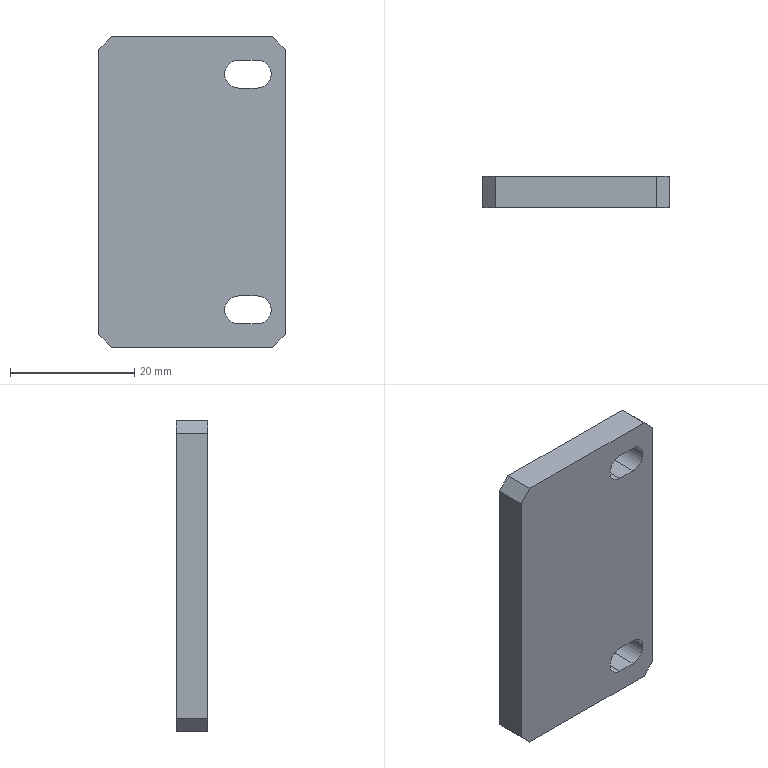Part | STEP file | P011002NM15-000 | 1 solid | 18 faces | box 30 x 5 x 50 mm | volume 7166 mm3 | plane 14 | cylinder 4 | commonest cylinder face diameters 4.5 x4
STEP:
#1=CARTESIAN_POINT('',(0.,0.,0.));
#2=DIRECTION('',(0.,0.,1.));
#3=DIRECTION('',(1.,0.,0.));
#4=AXIS2_PLACEMENT_3D('',#1,#2,#3);
#5=CARTESIAN_POINT('',(197.5,313.,-252.75));
#6=VERTEX_POINT('',#5);
#7=CARTESIAN_POINT('',(200.5,313.,-252.75));
#8=VERTEX_POINT('',#7);
#9=CARTESIAN_POINT('',(175.,313.,-252.75));
#10=DIRECTION('',(1.,0.,0.));
#11=VECTOR('',#10,1.);
#12=LINE('',#9,#11);
#13=CARTESIAN_POINT('',(175.,313.,-299.));
#14=DIRECTION('',(0.,-1.,0.));
#15=DIRECTION('',(0.,0.,-1.));
#16=AXIS2_PLACEMENT_3D('',#13,#14,#15);
#17=PLANE('',#16);
#18=CARTESIAN_POINT('',(-46.25,0.));
#19=DIRECTION('',(0.,1.));
#20=VECTOR('',#19,1.);
#21=LINE('',#18,#20);
#22=(GEOMETRIC_REPRESENTATION_CONTEXT(2)PARAMETRIC_REPRESENTATION_CONTEXT()REPRESENTATION_CONTEXT('',''));
#23=DEFINITIONAL_REPRESENTATION('',(#21),#22);
#24=PCURVE('',#17,#23);
#25=CARTESIAN_POINT('',(309.5,308.,-252.75));
#26=DIRECTION('',(0.,0.,1.));
#27=DIRECTION('',(1.,0.,0.));
#28=AXIS2_PLACEMENT_3D('',#25,#26,#27);
#29=PLANE('',#28);
#30=CARTESIAN_POINT('',(-134.5,5.));
#31=DIRECTION('',(1.,0.));
#32=VECTOR('',#31,1.);
#33=LINE('',#30,#32);
#34=(GEOMETRIC_REPRESENTATION_CONTEXT(2)PARAMETRIC_REPRESENTATION_CONTEXT()REPRESENTATION_CONTEXT('',''));
#35=DEFINITIONAL_REPRESENTATION('',(#33),#34);
#36=PCURVE('',#29,#35);
#37=SURFACE_CURVE('',#12,(#24,#36),.PCURVE_S1.);
#38=EDGE_CURVE('',#6,#8,#37,.T.);
#39=ORIENTED_EDGE('',*,*,#38,.F.);
#40=CARTESIAN_POINT('',(197.5,313.,-257.25));
#41=VERTEX_POINT('',#40);
#42=CARTESIAN_POINT('',(197.5,313.,-255.));
#43=DIRECTION('',(0.,-1.,0.));
#44=DIRECTION('',(0.,0.,-1.));
#45=AXIS2_PLACEMENT_3D('',#42,#43,#44);
#46=CIRCLE('',#45,2.25);
#47=CARTESIAN_POINT('',(-44.,22.5));
#48=DIRECTION('',(1.,0.));
#49=AXIS2_PLACEMENT_2D('',#47,#48);
#50=CIRCLE('',#49,2.25);
#51=(GEOMETRIC_REPRESENTATION_CONTEXT(2)PARAMETRIC_REPRESENTATION_CONTEXT()REPRESENTATION_CONTEXT('',''));
#52=DEFINITIONAL_REPRESENTATION('',(#50),#51);
#53=PCURVE('',#17,#52);
#54=CARTESIAN_POINT('',(197.5,327.267,-255.));
#55=DIRECTION('',(0.,-1.,0.));
#56=DIRECTION('',(1.,0.,0.));
#57=AXIS2_PLACEMENT_3D('',#54,#55,#56);
#58=CYLINDRICAL_SURFACE('',#57,2.25);
#59=CARTESIAN_POINT('',(-1.571,14.267));
#60=DIRECTION('',(1.,0.));
#61=VECTOR('',#60,1.);
#62=LINE('',#59,#61);
#63=(GEOMETRIC_REPRESENTATION_CONTEXT(2)PARAMETRIC_REPRESENTATION_CONTEXT()REPRESENTATION_CONTEXT('',''));
#64=DEFINITIONAL_REPRESENTATION('',(#62),#63);
#65=PCURVE('',#58,#64);
#66=SURFACE_CURVE('',#46,(#53,#65),.PCURVE_S1.);
#67=EDGE_CURVE('',#6,#41,#66,.T.);
#68=ORIENTED_EDGE('',*,*,#67,.T.);
#69=CARTESIAN_POINT('',(200.5,313.,-257.25));
#70=VERTEX_POINT('',#69);
#71=CARTESIAN_POINT('',(175.,313.,-257.25));
#72=DIRECTION('',(-1.,0.,0.));
#73=VECTOR('',#72,1.);
#74=LINE('',#71,#73);
#75=CARTESIAN_POINT('',(-41.75,0.));
#76=DIRECTION('',(0.,-1.));
#77=VECTOR('',#76,1.);
#78=LINE('',#75,#77);
#79=(GEOMETRIC_REPRESENTATION_CONTEXT(2)PARAMETRIC_REPRESENTATION_CONTEXT()REPRESENTATION_CONTEXT('',''));
#80=DEFINITIONAL_REPRESENTATION('',(#78),#79);
#81=PCURVE('',#17,#80);
#82=CARTESIAN_POINT('',(309.5,327.267,-257.25));
#83=DIRECTION('',(0.,0.,-1.));
#84=DIRECTION('',(-1.,0.,0.));
#85=AXIS2_PLACEMENT_3D('',#82,#83,#84);
#86=PLANE('',#85);
#87=CARTESIAN_POINT('',(134.5,-14.267));
#88=DIRECTION('',(1.,0.));
#89=VECTOR('',#88,1.);
#90=LINE('',#87,#89);
#91=(GEOMETRIC_REPRESENTATION_CONTEXT(2)PARAMETRIC_REPRESENTATION_CONTEXT()REPRESENTATION_CONTEXT('',''));
#92=DEFINITIONAL_REPRESENTATION('',(#90),#91);
#93=PCURVE('',#86,#92);
#94=SURFACE_CURVE('',#74,(#81,#93),.PCURVE_S1.);
#95=EDGE_CURVE('',#70,#41,#94,.T.);
#96=ORIENTED_EDGE('',*,*,#95,.F.);
#97=CARTESIAN_POINT('',(200.5,313.,-255.));
#98=DIRECTION('',(0.,-1.,0.));
#99=DIRECTION('',(0.,0.,-1.));
#100=AXIS2_PLACEMENT_3D('',#97,#98,#99);
#101=CIRCLE('',#100,2.25);
#102=CARTESIAN_POINT('',(-44.,25.5));
#103=DIRECTION('',(1.,0.));
#104=AXIS2_PLACEMENT_2D('',#102,#103);
#105=CIRCLE('',#104,2.25);
#106=(GEOMETRIC_REPRESENTATION_CONTEXT(2)PARAMETRIC_REPRESENTATION_CONTEXT()REPRESENTATION_CONTEXT('',''));
#107=DEFINITIONAL_REPRESENTATION('',(#105),#106);
#108=PCURVE('',#17,#107);
#109=CARTESIAN_POINT('',(200.5,327.267,-255.));
#110=DIRECTION('',(0.,-1.,0.));
#111=DIRECTION('',(-1.,0.,0.));
#112=AXIS2_PLACEMENT_3D('',#109,#110,#111);
#113=CYLINDRICAL_SURFACE('',#112,2.25);
#114=CARTESIAN_POINT('',(1.571,14.267));
#115=DIRECTION('',(1.,0.));
#116=VECTOR('',#115,1.);
#117=LINE('',#114,#116);
#118=(GEOMETRIC_REPRESENTATION_CONTEXT(2)PARAMETRIC_REPRESENTATION_CONTEXT()REPRESENTATION_CONTEXT('',''));
#119=DEFINITIONAL_REPRESENTATION('',(#117),#118);
#120=PCURVE('',#113,#119);
#121=SURFACE_CURVE('',#101,(#108,#120),.PCURVE_S1.);
#122=EDGE_CURVE('',#70,#8,#121,.T.);
#123=ORIENTED_EDGE('',*,*,#122,.T.);
#124=EDGE_LOOP('',(#39,#68,#96,#123));
#125=FACE_BOUND('',#124,.T.);
#126=CARTESIAN_POINT('',(205.,313.,-297.));
#127=VERTEX_POINT('',#126);
#128=CARTESIAN_POINT('',(205.,313.,-251.));
#129=VERTEX_POINT('',#128);
#130=CARTESIAN_POINT('',(205.,313.,-299.));
#131=DIRECTION('',(0.,0.,1.));
#132=VECTOR('',#131,1.);
#133=LINE('',#130,#132);
#134=CARTESIAN_POINT('',(0.,30.));
#135=DIRECTION('',(-1.,0.));
#136=VECTOR('',#135,1.);
#137=LINE('',#134,#136);
#138=(GEOMETRIC_REPRESENTATION_CONTEXT(2)PARAMETRIC_REPRESENTATION_CONTEXT()REPRESENTATION_CONTEXT('',''));
#139=DEFINITIONAL_REPRESENTATION('',(#137),#138);
#140=PCURVE('',#17,#139);
#141=CARTESIAN_POINT('',(205.,298.,-299.));
#142=DIRECTION('',(1.,0.,0.));
#143=DIRECTION('',(0.,0.,-1.));
#144=AXIS2_PLACEMENT_3D('',#141,#142,#143);
#145=PLANE('',#144);
#146=CARTESIAN_POINT('',(0.,15.));
#147=DIRECTION('',(-1.,0.));
#148=VECTOR('',#147,1.);
#149=LINE('',#146,#148);
#150=(GEOMETRIC_REPRESENTATION_CONTEXT(2)PARAMETRIC_REPRESENTATION_CONTEXT()REPRESENTATION_CONTEXT('',''));
#151=DEFINITIONAL_REPRESENTATION('',(#149),#150);
#152=PCURVE('',#145,#151);
#153=SURFACE_CURVE('',#133,(#140,#152),.PCURVE_S1.);
#154=EDGE_CURVE('',#127,#129,#153,.T.);
#155=ORIENTED_EDGE('',*,*,#154,.F.);
#156=CARTESIAN_POINT('',(203.,313.,-299.));
#157=VERTEX_POINT('',#156);
#158=CARTESIAN_POINT('',(189.,313.,-313.));
#159=DIRECTION('',(-0.7071,0.,-0.7071));
#160=VECTOR('',#159,1.);
#161=LINE('',#158,#160);
#162=CARTESIAN_POINT('',(14.,14.));
#163=DIRECTION('',(0.7071,-0.7071));
#164=VECTOR('',#163,1.);
#165=LINE('',#162,#164);
#166=(GEOMETRIC_REPRESENTATION_CONTEXT(2)PARAMETRIC_REPRESENTATION_CONTEXT()REPRESENTATION_CONTEXT('',''));
#167=DEFINITIONAL_REPRESENTATION('',(#165),#166);
#168=PCURVE('',#17,#167);
#169=CARTESIAN_POINT('',(205.,298.,-297.));
#170=DIRECTION('',(-0.7071,0.,0.7071));
#171=DIRECTION('',(0.7071,0.,0.7071));
#172=AXIS2_PLACEMENT_3D('',#169,#170,#171);
#173=PLANE('',#172);
#174=CARTESIAN_POINT('',(-22.627,15.));
#175=DIRECTION('',(-1.,0.));
#176=VECTOR('',#175,1.);
#177=LINE('',#174,#176);
#178=(GEOMETRIC_REPRESENTATION_CONTEXT(2)PARAMETRIC_REPRESENTATION_CONTEXT()REPRESENTATION_CONTEXT('',''));
#179=DEFINITIONAL_REPRESENTATION('',(#177),#178);
#180=PCURVE('',#173,#179);
#181=SURFACE_CURVE('',#161,(#168,#180),.PCURVE_S1.);
#182=EDGE_CURVE('',#127,#157,#181,.T.);
#183=ORIENTED_EDGE('',*,*,#182,.T.);
#184=CARTESIAN_POINT('',(177.,313.,-299.));
#185=VERTEX_POINT('',#184);
#186=CARTESIAN_POINT('',(175.,313.,-299.));
#187=DIRECTION('',(-1.,0.,0.));
#188=VECTOR('',#187,1.);
#189=LINE('',#186,#188);
#190=CARTESIAN_POINT('',(0.,0.));
#191=DIRECTION('',(0.,-1.));
#192=VECTOR('',#191,1.);
#193=LINE('',#190,#192);
#194=(GEOMETRIC_REPRESENTATION_CONTEXT(2)PARAMETRIC_REPRESENTATION_CONTEXT()REPRESENTATION_CONTEXT('',''));
#195=DEFINITIONAL_REPRESENTATION('',(#193),#194);
#196=PCURVE('',#17,#195);
#197=CARTESIAN_POINT('',(219.,548.,-299.));
#198=DIRECTION('',(0.,0.,-1.));
#199=DIRECTION('',(-1.,0.,0.));
#200=AXIS2_PLACEMENT_3D('',#197,#198,#199);
#201=PLANE('',#200);
#202=CARTESIAN_POINT('',(44.,-235.));
#203=DIRECTION('',(1.,0.));
#204=VECTOR('',#203,1.);
#205=LINE('',#202,#204);
#206=(GEOMETRIC_REPRESENTATION_CONTEXT(2)PARAMETRIC_REPRESENTATION_CONTEXT()REPRESENTATION_CONTEXT('',''));
#207=DEFINITIONAL_REPRESENTATION('',(#205),#206);
#208=PCURVE('',#201,#207);
#209=SURFACE_CURVE('',#189,(#196,#208),.PCURVE_S1.);
#210=EDGE_CURVE('',#157,#185,#209,.T.);
#211=ORIENTED_EDGE('',*,*,#210,.T.);
#212=CARTESIAN_POINT('',(175.,313.,-297.));
#213=VERTEX_POINT('',#212);
#214=CARTESIAN_POINT('',(176.,313.,-298.));
#215=DIRECTION('',(-0.7071,0.,0.7071));
#216=VECTOR('',#215,1.);
#217=LINE('',#214,#216);
#218=CARTESIAN_POINT('',(-1.,1.));
#219=DIRECTION('',(-0.7071,-0.7071));
#220=VECTOR('',#219,1.);
#221=LINE('',#218,#220);
#222=(GEOMETRIC_REPRESENTATION_CONTEXT(2)PARAMETRIC_REPRESENTATION_CONTEXT()REPRESENTATION_CONTEXT('',''));
#223=DEFINITIONAL_REPRESENTATION('',(#221),#222);
#224=PCURVE('',#17,#223);
#225=CARTESIAN_POINT('',(175.,548.,-297.));
#226=DIRECTION('',(0.7071,0.,0.7071));
#227=DIRECTION('',(0.7071,0.,-0.7071));
#228=AXIS2_PLACEMENT_3D('',#225,#226,#227);
#229=PLANE('',#228);
#230=CARTESIAN_POINT('',(1.414,-235.));
#231=DIRECTION('',(-1.,0.));
#232=VECTOR('',#231,1.);
#233=LINE('',#230,#232);
#234=(GEOMETRIC_REPRESENTATION_CONTEXT(2)PARAMETRIC_REPRESENTATION_CONTEXT()REPRESENTATION_CONTEXT('',''));
#235=DEFINITIONAL_REPRESENTATION('',(#233),#234);
#236=PCURVE('',#229,#235);
#237=SURFACE_CURVE('',#217,(#224,#236),.PCURVE_S1.);
#238=EDGE_CURVE('',#185,#213,#237,.T.);
#239=ORIENTED_EDGE('',*,*,#238,.T.);
#240=CARTESIAN_POINT('',(175.,313.,-251.));
#241=VERTEX_POINT('',#240);
#242=CARTESIAN_POINT('',(175.,313.,-299.));
#243=DIRECTION('',(0.,0.,1.));
#244=VECTOR('',#243,1.);
#245=LINE('',#242,#244);
#246=CARTESIAN_POINT('',(0.,0.));
#247=DIRECTION('',(-1.,0.));
#248=VECTOR('',#247,1.);
#249=LINE('',#246,#248);
#250=(GEOMETRIC_REPRESENTATION_CONTEXT(2)PARAMETRIC_REPRESENTATION_CONTEXT()REPRESENTATION_CONTEXT('',''));
#251=DEFINITIONAL_REPRESENTATION('',(#249),#250);
#252=PCURVE('',#17,#251);
#253=CARTESIAN_POINT('',(175.,548.,-69.));
#254=DIRECTION('',(-1.,0.,0.));
#255=DIRECTION('',(0.,0.,1.));
#256=AXIS2_PLACEMENT_3D('',#253,#254,#255);
#257=PLANE('',#256);
#258=CARTESIAN_POINT('',(-230.,-235.));
#259=DIRECTION('',(1.,0.));
#260=VECTOR('',#259,1.);
#261=LINE('',#258,#260);
#262=(GEOMETRIC_REPRESENTATION_CONTEXT(2)PARAMETRIC_REPRESENTATION_CONTEXT()REPRESENTATION_CONTEXT('',''));
#263=DEFINITIONAL_REPRESENTATION('',(#261),#262);
#264=PCURVE('',#257,#263);
#265=SURFACE_CURVE('',#245,(#252,#264),.PCURVE_S1.);
#266=EDGE_CURVE('',#213,#241,#265,.T.);
#267=ORIENTED_EDGE('',*,*,#266,.T.);
#268=CARTESIAN_POINT('',(177.,313.,-249.));
#269=VERTEX_POINT('',#268);
#270=CARTESIAN_POINT('',(151.,313.,-275.));
#271=DIRECTION('',(0.7071,0.,0.7071));
#272=VECTOR('',#271,1.);
#273=LINE('',#270,#272);
#274=CARTESIAN_POINT('',(-24.,-24.));
#275=DIRECTION('',(-0.7071,0.7071));
#276=VECTOR('',#275,1.);
#277=LINE('',#274,#276);
#278=(GEOMETRIC_REPRESENTATION_CONTEXT(2)PARAMETRIC_REPRESENTATION_CONTEXT()REPRESENTATION_CONTEXT('',''));
#279=DEFINITIONAL_REPRESENTATION('',(#277),#278);
#280=PCURVE('',#17,#279);
#281=CARTESIAN_POINT('',(175.,548.,-251.));
#282=DIRECTION('',(-0.7071,0.,0.7071));
#283=DIRECTION('',(0.7071,0.,0.7071));
#284=AXIS2_PLACEMENT_3D('',#281,#282,#283);
#285=PLANE('',#284);
#286=CARTESIAN_POINT('',(-33.941,-235.));
#287=DIRECTION('',(1.,0.));
#288=VECTOR('',#287,1.);
#289=LINE('',#286,#288);
#290=(GEOMETRIC_REPRESENTATION_CONTEXT(2)PARAMETRIC_REPRESENTATION_CONTEXT()REPRESENTATION_CONTEXT('',''));
#291=DEFINITIONAL_REPRESENTATION('',(#289),#290);
#292=PCURVE('',#285,#291);
#293=SURFACE_CURVE('',#273,(#280,#292),.PCURVE_S1.);
#294=EDGE_CURVE('',#241,#269,#293,.T.);
#295=ORIENTED_EDGE('',*,*,#294,.T.);
#296=CARTESIAN_POINT('',(203.,313.,-249.));
#297=VERTEX_POINT('',#296);
#298=CARTESIAN_POINT('',(175.,313.,-249.));
#299=DIRECTION('',(1.,0.,0.));
#300=VECTOR('',#299,1.);
#301=LINE('',#298,#300);
#302=CARTESIAN_POINT('',(-50.,0.));
#303=DIRECTION('',(0.,1.));
#304=VECTOR('',#303,1.);
#305=LINE('',#302,#304);
#306=(GEOMETRIC_REPRESENTATION_CONTEXT(2)PARAMETRIC_REPRESENTATION_CONTEXT()REPRESENTATION_CONTEXT('',''));
#307=DEFINITIONAL_REPRESENTATION('',(#305),#306);
#308=PCURVE('',#17,#307);
#309=CARTESIAN_POINT('',(175.,298.,-249.));
#310=DIRECTION('',(0.,0.,-1.));
#311=DIRECTION('',(1.,0.,0.));
#312=AXIS2_PLACEMENT_3D('',#309,#310,#311);
#313=PLANE('',#312);
#314=CARTESIAN_POINT('',(0.,-15.));
#315=DIRECTION('',(1.,0.));
#316=VECTOR('',#315,1.);
#317=LINE('',#314,#316);
#318=(GEOMETRIC_REPRESENTATION_CONTEXT(2)PARAMETRIC_REPRESENTATION_CONTEXT()REPRESENTATION_CONTEXT('',''));
#319=DEFINITIONAL_REPRESENTATION('',(#317),#318);
#320=PCURVE('',#313,#319);
#321=SURFACE_CURVE('',#301,(#308,#320),.PCURVE_S1.);
#322=EDGE_CURVE('',#269,#297,#321,.T.);
#323=ORIENTED_EDGE('',*,*,#322,.T.);
#324=CARTESIAN_POINT('',(214.,313.,-260.));
#325=DIRECTION('',(0.7071,0.,-0.7071));
#326=VECTOR('',#325,1.);
#327=LINE('',#324,#326);
#328=CARTESIAN_POINT('',(-39.,39.));
#329=DIRECTION('',(0.7071,0.7071));
#330=VECTOR('',#329,1.);
#331=LINE('',#328,#330);
#332=(GEOMETRIC_REPRESENTATION_CONTEXT(2)PARAMETRIC_REPRESENTATION_CONTEXT()REPRESENTATION_CONTEXT('',''));
#333=DEFINITIONAL_REPRESENTATION('',(#331),#332);
#334=PCURVE('',#17,#333);
#335=CARTESIAN_POINT('',(205.,298.,-251.));
#336=DIRECTION('',(0.7071,0.,0.7071));
#337=DIRECTION('',(0.7071,0.,-0.7071));
#338=AXIS2_PLACEMENT_3D('',#335,#336,#337);
#339=PLANE('',#338);
#340=CARTESIAN_POINT('',(12.728,15.));
#341=DIRECTION('',(1.,0.));
#342=VECTOR('',#341,1.);
#343=LINE('',#340,#342);
#344=(GEOMETRIC_REPRESENTATION_CONTEXT(2)PARAMETRIC_REPRESENTATION_CONTEXT()REPRESENTATION_CONTEXT('',''));
#345=DEFINITIONAL_REPRESENTATION('',(#343),#344);
#346=PCURVE('',#339,#345);
#347=SURFACE_CURVE('',#327,(#334,#346),.PCURVE_S1.);
#348=EDGE_CURVE('',#297,#129,#347,.T.);
#349=ORIENTED_EDGE('',*,*,#348,.T.);
#350=EDGE_LOOP('',(#155,#183,#211,#239,#267,#295,#323,#349));
#351=FACE_BOUND('',#350,.T.);
#352=CARTESIAN_POINT('',(197.5,313.,-290.75));
#353=VERTEX_POINT('',#352);
#354=CARTESIAN_POINT('',(200.5,313.,-290.75));
#355=VERTEX_POINT('',#354);
#356=CARTESIAN_POINT('',(175.,313.,-290.75));
#357=DIRECTION('',(1.,0.,0.));
#358=VECTOR('',#357,1.);
#359=LINE('',#356,#358);
#360=CARTESIAN_POINT('',(-8.25,0.));
#361=DIRECTION('',(0.,1.));
#362=VECTOR('',#361,1.);
#363=LINE('',#360,#362);
#364=(GEOMETRIC_REPRESENTATION_CONTEXT(2)PARAMETRIC_REPRESENTATION_CONTEXT()REPRESENTATION_CONTEXT('',''));
#365=DEFINITIONAL_REPRESENTATION('',(#363),#364);
#366=PCURVE('',#17,#365);
#367=CARTESIAN_POINT('',(309.5,327.267,-290.75));
#368=DIRECTION('',(0.,0.,1.));
#369=DIRECTION('',(-1.,0.,0.));
#370=AXIS2_PLACEMENT_3D('',#367,#368,#369);
#371=PLANE('',#370);
#372=CARTESIAN_POINT('',(134.5,14.267));
#373=DIRECTION('',(-1.,0.));
#374=VECTOR('',#373,1.);
#375=LINE('',#372,#374);
#376=(GEOMETRIC_REPRESENTATION_CONTEXT(2)PARAMETRIC_REPRESENTATION_CONTEXT()REPRESENTATION_CONTEXT('',''));
#377=DEFINITIONAL_REPRESENTATION('',(#375),#376);
#378=PCURVE('',#371,#377);
#379=SURFACE_CURVE('',#359,(#366,#378),.PCURVE_S1.);
#380=EDGE_CURVE('',#353,#355,#379,.T.);
#381=ORIENTED_EDGE('',*,*,#380,.F.);
#382=CARTESIAN_POINT('',(197.5,313.,-295.25));
#383=VERTEX_POINT('',#382);
#384=CARTESIAN_POINT('',(197.5,313.,-293.));
#385=DIRECTION('',(0.,-1.,0.));
#386=DIRECTION('',(0.,0.,-1.));
#387=AXIS2_PLACEMENT_3D('',#384,#385,#386);
#388=CIRCLE('',#387,2.25);
#389=CARTESIAN_POINT('',(-6.,22.5));
#390=DIRECTION('',(1.,0.));
#391=AXIS2_PLACEMENT_2D('',#389,#390);
#392=CIRCLE('',#391,2.25);
#393=(GEOMETRIC_REPRESENTATION_CONTEXT(2)PARAMETRIC_REPRESENTATION_CONTEXT()REPRESENTATION_CONTEXT('',''));
#394=DEFINITIONAL_REPRESENTATION('',(#392),#393);
#395=PCURVE('',#17,#394);
#396=CARTESIAN_POINT('',(197.5,327.267,-293.));
#397=DIRECTION('',(0.,-1.,0.));
#398=DIRECTION('',(1.,0.,0.));
#399=AXIS2_PLACEMENT_3D('',#396,#397,#398);
#400=CYLINDRICAL_SURFACE('',#399,2.25);
#401=CARTESIAN_POINT('',(-1.571,14.267));
#402=DIRECTION('',(1.,0.));
#403=VECTOR('',#402,1.);
#404=LINE('',#401,#403);
#405=(GEOMETRIC_REPRESENTATION_CONTEXT(2)PARAMETRIC_REPRESENTATION_CONTEXT()REPRESENTATION_CONTEXT('',''));
#406=DEFINITIONAL_REPRESENTATION('',(#404),#405);
#407=PCURVE('',#400,#406);
#408=SURFACE_CURVE('',#388,(#395,#407),.PCURVE_S1.);
#409=EDGE_CURVE('',#353,#383,#408,.T.);
#410=ORIENTED_EDGE('',*,*,#409,.T.);
#411=CARTESIAN_POINT('',(200.5,313.,-295.25));
#412=VERTEX_POINT('',#411);
#413=CARTESIAN_POINT('',(175.,313.,-295.25));
#414=DIRECTION('',(-1.,0.,0.));
#415=VECTOR('',#414,1.);
#416=LINE('',#413,#415);
#417=CARTESIAN_POINT('',(-3.75,0.));
#418=DIRECTION('',(0.,-1.));
#419=VECTOR('',#418,1.);
#420=LINE('',#417,#419);
#421=(GEOMETRIC_REPRESENTATION_CONTEXT(2)PARAMETRIC_REPRESENTATION_CONTEXT()REPRESENTATION_CONTEXT('',''));
#422=DEFINITIONAL_REPRESENTATION('',(#420),#421);
#423=PCURVE('',#17,#422);
#424=CARTESIAN_POINT('',(309.5,308.,-295.25));
#425=DIRECTION('',(0.,0.,-1.));
#426=DIRECTION('',(1.,0.,0.));
#427=AXIS2_PLACEMENT_3D('',#424,#425,#426);
#428=PLANE('',#427);
#429=CARTESIAN_POINT('',(-134.5,-5.));
#430=DIRECTION('',(-1.,0.));
#431=VECTOR('',#430,1.);
#432=LINE('',#429,#431);
#433=(GEOMETRIC_REPRESENTATION_CONTEXT(2)PARAMETRIC_REPRESENTATION_CONTEXT()REPRESENTATION_CONTEXT('',''));
#434=DEFINITIONAL_REPRESENTATION('',(#432),#433);
#435=PCURVE('',#428,#434);
#436=SURFACE_CURVE('',#416,(#423,#435),.PCURVE_S1.);
#437=EDGE_CURVE('',#412,#383,#436,.T.);
#438=ORIENTED_EDGE('',*,*,#437,.F.);
#439=CARTESIAN_POINT('',(200.5,313.,-293.));
#440=DIRECTION('',(0.,-1.,0.));
#441=DIRECTION('',(0.,0.,-1.));
#442=AXIS2_PLACEMENT_3D('',#439,#440,#441);
#443=CIRCLE('',#442,2.25);
#444=CARTESIAN_POINT('',(-6.,25.5));
#445=DIRECTION('',(1.,0.));
#446=AXIS2_PLACEMENT_2D('',#444,#445);
#447=CIRCLE('',#446,2.25);
#448=(GEOMETRIC_REPRESENTATION_CONTEXT(2)PARAMETRIC_REPRESENTATION_CONTEXT()REPRESENTATION_CONTEXT('',''));
#449=DEFINITIONAL_REPRESENTATION('',(#447),#448);
#450=PCURVE('',#17,#449);
#451=CARTESIAN_POINT('',(200.5,327.267,-293.));
#452=DIRECTION('',(0.,-1.,0.));
#453=DIRECTION('',(-1.,0.,0.));
#454=AXIS2_PLACEMENT_3D('',#451,#452,#453);
#455=CYLINDRICAL_SURFACE('',#454,2.25);
#456=CARTESIAN_POINT('',(1.571,14.267));
#457=DIRECTION('',(1.,0.));
#458=VECTOR('',#457,1.);
#459=LINE('',#456,#458);
#460=(GEOMETRIC_REPRESENTATION_CONTEXT(2)PARAMETRIC_REPRESENTATION_CONTEXT()REPRESENTATION_CONTEXT('',''));
#461=DEFINITIONAL_REPRESENTATION('',(#459),#460);
#462=PCURVE('',#455,#461);
#463=SURFACE_CURVE('',#443,(#450,#462),.PCURVE_S1.);
#464=EDGE_CURVE('',#412,#355,#463,.T.);
#465=ORIENTED_EDGE('',*,*,#464,.T.);
#466=EDGE_LOOP('',(#381,#410,#438,#465));
#467=FACE_BOUND('',#466,.T.);
#468=ADVANCED_FACE('',(#125,#351,#467),#17,.F.);
#469=CARTESIAN_POINT('',(200.5,308.,-290.75));
#470=VERTEX_POINT('',#469);
#471=CARTESIAN_POINT('',(197.5,308.,-290.75));
#472=VERTEX_POINT('',#471);
#473=CARTESIAN_POINT('',(309.5,308.,-290.75));
#474=DIRECTION('',(-1.,0.,0.));
#475=VECTOR('',#474,1.);
#476=LINE('',#473,#475);
#477=CARTESIAN_POINT('',(219.,308.,-69.));
#478=DIRECTION('',(0.,-1.,0.));
#479=DIRECTION('',(0.,0.,1.));
#480=AXIS2_PLACEMENT_3D('',#477,#478,#479);
#481=PLANE('',#480);
#482=CARTESIAN_POINT('',(-221.75,-90.5));
#483=DIRECTION('',(0.,1.));
#484=VECTOR('',#483,1.);
#485=LINE('',#482,#484);
#486=(GEOMETRIC_REPRESENTATION_CONTEXT(2)PARAMETRIC_REPRESENTATION_CONTEXT()REPRESENTATION_CONTEXT('',''));
#487=DEFINITIONAL_REPRESENTATION('',(#485),#486);
#488=PCURVE('',#481,#487);
#489=CARTESIAN_POINT('',(0.,19.267));
#490=DIRECTION('',(1.,0.));
#491=VECTOR('',#490,1.);
#492=LINE('',#489,#491);
#493=(GEOMETRIC_REPRESENTATION_CONTEXT(2)PARAMETRIC_REPRESENTATION_CONTEXT()REPRESENTATION_CONTEXT('',''));
#494=DEFINITIONAL_REPRESENTATION('',(#492),#493);
#495=PCURVE('',#371,#494);
#496=SURFACE_CURVE('',#476,(#488,#495),.PCURVE_S1.);
#497=EDGE_CURVE('',#470,#472,#496,.T.);
#498=ORIENTED_EDGE('',*,*,#497,.F.);
#499=CARTESIAN_POINT('',(200.5,308.,-295.25));
#500=VERTEX_POINT('',#499);
#501=CARTESIAN_POINT('',(200.5,308.,-293.));
#502=DIRECTION('',(0.,1.,0.));
#503=DIRECTION('',(1.,0.,0.));
#504=AXIS2_PLACEMENT_3D('',#501,#502,#503);
#505=CIRCLE('',#504,2.25);
#506=CARTESIAN_POINT('',(-224.,16.25));
#507=CARTESIAN_POINT('',(-227.897,16.25));
#508=CARTESIAN_POINT('',(-225.949,19.625));
#509=CARTESIAN_POINT('',(-224.,23.));
#510=CARTESIAN_POINT('',(-222.051,19.625));
#511=CARTESIAN_POINT('',(-220.103,16.25));
#512=CARTESIAN_POINT('',(-224.,16.25));
#513=(BOUNDED_CURVE()B_SPLINE_CURVE(2,(#506,#507,#508,#509,#510,#511,#512),.UNSPECIFIED.,.T.,.F.)B_SPLINE_CURVE_WITH_KNOTS((1,2,2,2,2,1),(-2.094,0.,2.094,4.189,6.283,8.378),.UNSPECIFIED.)CURVE()GEOMETRIC_REPRESENTATION_ITEM()RATIONAL_B_SPLINE_CURVE((1.,0.5,1.,0.5,1.,0.5,1.))REPRESENTATION_ITEM(''));
#514=(GEOMETRIC_REPRESENTATION_CONTEXT(2)PARAMETRIC_REPRESENTATION_CONTEXT()REPRESENTATION_CONTEXT('',''));
#515=DEFINITIONAL_REPRESENTATION('',(#513),#514);
#516=PCURVE('',#481,#515);
#517=CARTESIAN_POINT('',(9.425,19.267));
#518=DIRECTION('',(-1.,0.));
#519=VECTOR('',#518,1.);
#520=LINE('',#517,#519);
#521=(GEOMETRIC_REPRESENTATION_CONTEXT(2)PARAMETRIC_REPRESENTATION_CONTEXT()REPRESENTATION_CONTEXT('',''));
#522=DEFINITIONAL_REPRESENTATION('',(#520),#521);
#523=PCURVE('',#455,#522);
#524=SURFACE_CURVE('',#505,(#516,#523),.PCURVE_S1.);
#525=EDGE_CURVE('',#470,#500,#524,.T.);
#526=ORIENTED_EDGE('',*,*,#525,.T.);
#527=CARTESIAN_POINT('',(197.5,308.,-295.25));
#528=VERTEX_POINT('',#527);
#529=CARTESIAN_POINT('',(309.5,308.,-295.25));
#530=DIRECTION('',(-1.,0.,0.));
#531=VECTOR('',#530,1.);
#532=LINE('',#529,#531);
#533=CARTESIAN_POINT('',(-226.25,-90.5));
#534=DIRECTION('',(0.,1.));
#535=VECTOR('',#534,1.);
#536=LINE('',#533,#535);
#537=(GEOMETRIC_REPRESENTATION_CONTEXT(2)PARAMETRIC_REPRESENTATION_CONTEXT()REPRESENTATION_CONTEXT('',''));
#538=DEFINITIONAL_REPRESENTATION('',(#536),#537);
#539=PCURVE('',#481,#538);
#540=CARTESIAN_POINT('',(0.,0.));
#541=DIRECTION('',(-1.,0.));
#542=VECTOR('',#541,1.);
#543=LINE('',#540,#542);
#544=(GEOMETRIC_REPRESENTATION_CONTEXT(2)PARAMETRIC_REPRESENTATION_CONTEXT()REPRESENTATION_CONTEXT('',''));
#545=DEFINITIONAL_REPRESENTATION('',(#543),#544);
#546=PCURVE('',#428,#545);
#547=SURFACE_CURVE('',#532,(#539,#546),.PCURVE_S1.);
#548=EDGE_CURVE('',#500,#528,#547,.T.);
#549=ORIENTED_EDGE('',*,*,#548,.T.);
#550=CARTESIAN_POINT('',(197.5,308.,-293.));
#551=DIRECTION('',(0.,-1.,0.));
#552=DIRECTION('',(-1.,0.,0.));
#553=AXIS2_PLACEMENT_3D('',#550,#551,#552);
#554=CIRCLE('',#553,2.25);
#555=CARTESIAN_POINT('',(-224.,21.5));
#556=DIRECTION('',(0.,1.));
#557=AXIS2_PLACEMENT_2D('',#555,#556);
#558=CIRCLE('',#557,2.25);
#559=(GEOMETRIC_REPRESENTATION_CONTEXT(2)PARAMETRIC_REPRESENTATION_CONTEXT()REPRESENTATION_CONTEXT('',''));
#560=DEFINITIONAL_REPRESENTATION('',(#558),#559);
#561=PCURVE('',#481,#560);
#562=CARTESIAN_POINT('',(-3.142,19.267));
#563=DIRECTION('',(1.,0.));
#564=VECTOR('',#563,1.);
#565=LINE('',#562,#564);
#566=(GEOMETRIC_REPRESENTATION_CONTEXT(2)PARAMETRIC_REPRESENTATION_CONTEXT()REPRESENTATION_CONTEXT('',''));
#567=DEFINITIONAL_REPRESENTATION('',(#565),#566);
#568=PCURVE('',#400,#567);
#569=SURFACE_CURVE('',#554,(#561,#568),.PCURVE_S1.);
#570=EDGE_CURVE('',#472,#528,#569,.T.);
#571=ORIENTED_EDGE('',*,*,#570,.F.);
#572=EDGE_LOOP('',(#498,#526,#549,#571));
#573=FACE_BOUND('',#572,.T.);
#574=CARTESIAN_POINT('',(177.,308.,-299.));
#575=VERTEX_POINT('',#574);
#576=CARTESIAN_POINT('',(203.,308.,-299.));
#577=VERTEX_POINT('',#576);
#578=CARTESIAN_POINT('',(219.,308.,-299.));
#579=DIRECTION('',(1.,0.,0.));
#580=VECTOR('',#579,1.);
#581=LINE('',#578,#580);
#582=CARTESIAN_POINT('',(-230.,0.));
#583=DIRECTION('',(0.,-1.));
#584=VECTOR('',#583,1.);
#585=LINE('',#582,#584);
#586=(GEOMETRIC_REPRESENTATION_CONTEXT(2)PARAMETRIC_REPRESENTATION_CONTEXT()REPRESENTATION_CONTEXT('',''));
#587=DEFINITIONAL_REPRESENTATION('',(#585),#586);
#588=PCURVE('',#481,#587);
#589=CARTESIAN_POINT('',(0.,-240.));
#590=DIRECTION('',(-1.,0.));
#591=VECTOR('',#590,1.);
#592=LINE('',#589,#591);
#593=(GEOMETRIC_REPRESENTATION_CONTEXT(2)PARAMETRIC_REPRESENTATION_CONTEXT()REPRESENTATION_CONTEXT('',''));
#594=DEFINITIONAL_REPRESENTATION('',(#592),#593);
#595=PCURVE('',#201,#594);
#596=SURFACE_CURVE('',#581,(#588,#595),.PCURVE_S1.);
#597=EDGE_CURVE('',#575,#577,#596,.T.);
#598=ORIENTED_EDGE('',*,*,#597,.T.);
#599=CARTESIAN_POINT('',(205.,308.,-297.));
#600=VERTEX_POINT('',#599);
#601=CARTESIAN_POINT('',(326.,308.,-176.));
#602=DIRECTION('',(0.7071,0.,0.7071));
#603=VECTOR('',#602,1.);
#604=LINE('',#601,#603);
#605=CARTESIAN_POINT('',(-107.,-107.));
#606=DIRECTION('',(0.7071,-0.7071));
#607=VECTOR('',#606,1.);
#608=LINE('',#605,#607);
#609=(GEOMETRIC_REPRESENTATION_CONTEXT(2)PARAMETRIC_REPRESENTATION_CONTEXT()REPRESENTATION_CONTEXT('',''));
#610=DEFINITIONAL_REPRESENTATION('',(#608),#609);
#611=PCURVE('',#481,#610);
#612=CARTESIAN_POINT('',(171.12,10.));
#613=DIRECTION('',(1.,0.));
#614=VECTOR('',#613,1.);
#615=LINE('',#612,#614);
#616=(GEOMETRIC_REPRESENTATION_CONTEXT(2)PARAMETRIC_REPRESENTATION_CONTEXT()REPRESENTATION_CONTEXT('',''));
#617=DEFINITIONAL_REPRESENTATION('',(#615),#616);
#618=PCURVE('',#173,#617);
#619=SURFACE_CURVE('',#604,(#611,#618),.PCURVE_S1.);
#620=EDGE_CURVE('',#577,#600,#619,.T.);
#621=ORIENTED_EDGE('',*,*,#620,.T.);
#622=CARTESIAN_POINT('',(205.,308.,-251.));
#623=VERTEX_POINT('',#622);
#624=CARTESIAN_POINT('',(205.,308.,-69.));
#625=DIRECTION('',(0.,0.,1.));
#626=VECTOR('',#625,1.);
#627=LINE('',#624,#626);
#628=CARTESIAN_POINT('',(0.,14.));
#629=DIRECTION('',(1.,0.));
#630=VECTOR('',#629,1.);
#631=LINE('',#628,#630);
#632=(GEOMETRIC_REPRESENTATION_CONTEXT(2)PARAMETRIC_REPRESENTATION_CONTEXT()REPRESENTATION_CONTEXT('',''));
#633=DEFINITIONAL_REPRESENTATION('',(#631),#632);
#634=PCURVE('',#481,#633);
#635=CARTESIAN_POINT('',(-230.,10.));
#636=DIRECTION('',(-1.,0.));
#637=VECTOR('',#636,1.);
#638=LINE('',#635,#637);
#639=(GEOMETRIC_REPRESENTATION_CONTEXT(2)PARAMETRIC_REPRESENTATION_CONTEXT()REPRESENTATION_CONTEXT('',''));
#640=DEFINITIONAL_REPRESENTATION('',(#638),#639);
#641=PCURVE('',#145,#640);
#642=SURFACE_CURVE('',#627,(#634,#641),.PCURVE_S1.);
#643=EDGE_CURVE('',#600,#623,#642,.T.);
#644=ORIENTED_EDGE('',*,*,#643,.T.);
#645=CARTESIAN_POINT('',(203.,308.,-249.));
#646=VERTEX_POINT('',#645);
#647=CARTESIAN_POINT('',(121.,308.,-167.));
#648=DIRECTION('',(-0.7071,0.,0.7071));
#649=VECTOR('',#648,1.);
#650=LINE('',#647,#649);
#651=CARTESIAN_POINT('',(-98.,98.));
#652=DIRECTION('',(0.7071,0.7071));
#653=VECTOR('',#652,1.);
#654=LINE('',#651,#653);
#655=(GEOMETRIC_REPRESENTATION_CONTEXT(2)PARAMETRIC_REPRESENTATION_CONTEXT()REPRESENTATION_CONTEXT('',''));
#656=DEFINITIONAL_REPRESENTATION('',(#654),#655);
#657=PCURVE('',#481,#656);
#658=CARTESIAN_POINT('',(-118.794,10.));
#659=DIRECTION('',(-1.,0.));
#660=VECTOR('',#659,1.);
#661=LINE('',#658,#660);
#662=(GEOMETRIC_REPRESENTATION_CONTEXT(2)PARAMETRIC_REPRESENTATION_CONTEXT()REPRESENTATION_CONTEXT('',''));
#663=DEFINITIONAL_REPRESENTATION('',(#661),#662);
#664=PCURVE('',#339,#663);
#665=SURFACE_CURVE('',#650,(#657,#664),.PCURVE_S1.);
#666=EDGE_CURVE('',#623,#646,#665,.T.);
#667=ORIENTED_EDGE('',*,*,#666,.T.);
#668=CARTESIAN_POINT('',(177.,308.,-249.));
#669=VERTEX_POINT('',#668);
#670=CARTESIAN_POINT('',(219.,308.,-249.));
#671=DIRECTION('',(-1.,0.,0.));
#672=VECTOR('',#671,1.);
#673=LINE('',#670,#672);
#674=CARTESIAN_POINT('',(-180.,0.));
#675=DIRECTION('',(0.,1.));
#676=VECTOR('',#675,1.);
#677=LINE('',#674,#676);
#678=(GEOMETRIC_REPRESENTATION_CONTEXT(2)PARAMETRIC_REPRESENTATION_CONTEXT()REPRESENTATION_CONTEXT('',''));
#679=DEFINITIONAL_REPRESENTATION('',(#677),#678);
#680=PCURVE('',#481,#679);
#681=CARTESIAN_POINT('',(44.,-10.));
#682=DIRECTION('',(-1.,0.));
#683=VECTOR('',#682,1.);
#684=LINE('',#681,#683);
#685=(GEOMETRIC_REPRESENTATION_CONTEXT(2)PARAMETRIC_REPRESENTATION_CONTEXT()REPRESENTATION_CONTEXT('',''));
#686=DEFINITIONAL_REPRESENTATION('',(#684),#685);
#687=PCURVE('',#313,#686);
#688=SURFACE_CURVE('',#673,(#680,#687),.PCURVE_S1.);
#689=EDGE_CURVE('',#646,#669,#688,.T.);
#690=ORIENTED_EDGE('',*,*,#689,.T.);
#691=CARTESIAN_POINT('',(175.,308.,-251.));
#692=VERTEX_POINT('',#691);
#693=CARTESIAN_POINT('',(288.,308.,-138.));
#694=DIRECTION('',(-0.7071,0.,-0.7071));
#695=VECTOR('',#694,1.);
#696=LINE('',#693,#695);
#697=CARTESIAN_POINT('',(-69.,-69.));
#698=DIRECTION('',(-0.7071,0.7071));
#699=VECTOR('',#698,1.);
#700=LINE('',#697,#699);
#701=(GEOMETRIC_REPRESENTATION_CONTEXT(2)PARAMETRIC_REPRESENTATION_CONTEXT()REPRESENTATION_CONTEXT('',''));
#702=DEFINITIONAL_REPRESENTATION('',(#700),#701);
#703=PCURVE('',#481,#702);
#704=CARTESIAN_POINT('',(159.806,-240.));
#705=DIRECTION('',(-1.,0.));
#706=VECTOR('',#705,1.);
#707=LINE('',#704,#706);
#708=(GEOMETRIC_REPRESENTATION_CONTEXT(2)PARAMETRIC_REPRESENTATION_CONTEXT()REPRESENTATION_CONTEXT('',''));
#709=DEFINITIONAL_REPRESENTATION('',(#707),#708);
#710=PCURVE('',#285,#709);
#711=SURFACE_CURVE('',#696,(#703,#710),.PCURVE_S1.);
#712=EDGE_CURVE('',#669,#692,#711,.T.);
#713=ORIENTED_EDGE('',*,*,#712,.T.);
#714=CARTESIAN_POINT('',(175.,308.,-297.));
#715=VERTEX_POINT('',#714);
#716=CARTESIAN_POINT('',(175.,308.,-69.));
#717=DIRECTION('',(0.,0.,1.));
#718=VECTOR('',#717,1.);
#719=LINE('',#716,#718);
#720=CARTESIAN_POINT('',(0.,44.));
#721=DIRECTION('',(1.,0.));
#722=VECTOR('',#721,1.);
#723=LINE('',#720,#722);
#724=(GEOMETRIC_REPRESENTATION_CONTEXT(2)PARAMETRIC_REPRESENTATION_CONTEXT()REPRESENTATION_CONTEXT('',''));
#725=DEFINITIONAL_REPRESENTATION('',(#723),#724);
#726=PCURVE('',#481,#725);
#727=CARTESIAN_POINT('',(0.,-240.));
#728=DIRECTION('',(1.,0.));
#729=VECTOR('',#728,1.);
#730=LINE('',#727,#729);
#731=(GEOMETRIC_REPRESENTATION_CONTEXT(2)PARAMETRIC_REPRESENTATION_CONTEXT()REPRESENTATION_CONTEXT('',''));
#732=DEFINITIONAL_REPRESENTATION('',(#730),#731);
#733=PCURVE('',#257,#732);
#734=SURFACE_CURVE('',#719,(#726,#733),.PCURVE_S1.);
#735=EDGE_CURVE('',#715,#692,#734,.T.);
#736=ORIENTED_EDGE('',*,*,#735,.F.);
#737=CARTESIAN_POINT('',(83.,308.,-205.));
#738=DIRECTION('',(0.7071,0.,-0.7071));
#739=VECTOR('',#738,1.);
#740=LINE('',#737,#739);
#741=CARTESIAN_POINT('',(-136.,136.));
#742=DIRECTION('',(-0.7071,-0.7071));
#743=VECTOR('',#742,1.);
#744=LINE('',#741,#743);
#745=(GEOMETRIC_REPRESENTATION_CONTEXT(2)PARAMETRIC_REPRESENTATION_CONTEXT()REPRESENTATION_CONTEXT('',''));
#746=DEFINITIONAL_REPRESENTATION('',(#744),#745);
#747=PCURVE('',#481,#746);
#748=CARTESIAN_POINT('',(-130.108,-240.));
#749=DIRECTION('',(1.,0.));
#750=VECTOR('',#749,1.);
#751=LINE('',#748,#750);
#752=(GEOMETRIC_REPRESENTATION_CONTEXT(2)PARAMETRIC_REPRESENTATION_CONTEXT()REPRESENTATION_CONTEXT('',''));
#753=DEFINITIONAL_REPRESENTATION('',(#751),#752);
#754=PCURVE('',#229,#753);
#755=SURFACE_CURVE('',#740,(#747,#754),.PCURVE_S1.);
#756=EDGE_CURVE('',#715,#575,#755,.T.);
#757=ORIENTED_EDGE('',*,*,#756,.T.);
#758=EDGE_LOOP('',(#598,#621,#644,#667,#690,#713,#736,#757));
#759=FACE_BOUND('',#758,.T.);
#760=CARTESIAN_POINT('',(200.5,308.,-257.25));
#761=VERTEX_POINT('',#760);
#762=CARTESIAN_POINT('',(200.5,308.,-252.75));
#763=VERTEX_POINT('',#762);
#764=CARTESIAN_POINT('',(200.5,308.,-255.));
#765=DIRECTION('',(0.,-1.,0.));
#766=DIRECTION('',(1.,0.,0.));
#767=AXIS2_PLACEMENT_3D('',#764,#765,#766);
#768=CIRCLE('',#767,2.25);
#769=CARTESIAN_POINT('',(-186.,18.5));
#770=DIRECTION('',(0.,-1.));
#771=AXIS2_PLACEMENT_2D('',#769,#770);
#772=CIRCLE('',#771,2.25);
#773=(GEOMETRIC_REPRESENTATION_CONTEXT(2)PARAMETRIC_REPRESENTATION_CONTEXT()REPRESENTATION_CONTEXT('',''));
#774=DEFINITIONAL_REPRESENTATION('',(#772),#773);
#775=PCURVE('',#481,#774);
#776=CARTESIAN_POINT('',(-3.142,19.267));
#777=DIRECTION('',(1.,0.));
#778=VECTOR('',#777,1.);
#779=LINE('',#776,#778);
#780=(GEOMETRIC_REPRESENTATION_CONTEXT(2)PARAMETRIC_REPRESENTATION_CONTEXT()REPRESENTATION_CONTEXT('',''));
#781=DEFINITIONAL_REPRESENTATION('',(#779),#780);
#782=PCURVE('',#113,#781);
#783=SURFACE_CURVE('',#768,(#775,#782),.PCURVE_S1.);
#784=EDGE_CURVE('',#761,#763,#783,.T.);
#785=ORIENTED_EDGE('',*,*,#784,.F.);
#786=CARTESIAN_POINT('',(197.5,308.,-257.25));
#787=VERTEX_POINT('',#786);
#788=CARTESIAN_POINT('',(309.5,308.,-257.25));
#789=DIRECTION('',(-1.,0.,0.));
#790=VECTOR('',#789,1.);
#791=LINE('',#788,#790);
#792=CARTESIAN_POINT('',(-188.25,-90.5));
#793=DIRECTION('',(0.,1.));
#794=VECTOR('',#793,1.);
#795=LINE('',#792,#794);
#796=(GEOMETRIC_REPRESENTATION_CONTEXT(2)PARAMETRIC_REPRESENTATION_CONTEXT()REPRESENTATION_CONTEXT('',''));
#797=DEFINITIONAL_REPRESENTATION('',(#795),#796);
#798=PCURVE('',#481,#797);
#799=CARTESIAN_POINT('',(0.,-19.267));
#800=DIRECTION('',(1.,0.));
#801=VECTOR('',#800,1.);
#802=LINE('',#799,#801);
#803=(GEOMETRIC_REPRESENTATION_CONTEXT(2)PARAMETRIC_REPRESENTATION_CONTEXT()REPRESENTATION_CONTEXT('',''));
#804=DEFINITIONAL_REPRESENTATION('',(#802),#803);
#805=PCURVE('',#86,#804);
#806=SURFACE_CURVE('',#791,(#798,#805),.PCURVE_S1.);
#807=EDGE_CURVE('',#761,#787,#806,.T.);
#808=ORIENTED_EDGE('',*,*,#807,.T.);
#809=CARTESIAN_POINT('',(197.5,308.,-252.75));
#810=VERTEX_POINT('',#809);
#811=CARTESIAN_POINT('',(197.5,308.,-255.));
#812=DIRECTION('',(0.,1.,0.));
#813=DIRECTION('',(-1.,0.,0.));
#814=AXIS2_PLACEMENT_3D('',#811,#812,#813);
#815=CIRCLE('',#814,2.25);
#816=CARTESIAN_POINT('',(-186.,23.75));
#817=CARTESIAN_POINT('',(-182.103,23.75));
#818=CARTESIAN_POINT('',(-184.051,20.375));
#819=CARTESIAN_POINT('',(-186.,17.));
#820=CARTESIAN_POINT('',(-187.949,20.375));
#821=CARTESIAN_POINT('',(-189.897,23.75));
#822=CARTESIAN_POINT('',(-186.,23.75));
#823=(BOUNDED_CURVE()B_SPLINE_CURVE(2,(#816,#817,#818,#819,#820,#821,#822),.UNSPECIFIED.,.T.,.F.)B_SPLINE_CURVE_WITH_KNOTS((1,2,2,2,2,1),(-2.094,0.,2.094,4.189,6.283,8.378),.UNSPECIFIED.)CURVE()GEOMETRIC_REPRESENTATION_ITEM()RATIONAL_B_SPLINE_CURVE((1.,0.5,1.,0.5,1.,0.5,1.))REPRESENTATION_ITEM(''));
#824=(GEOMETRIC_REPRESENTATION_CONTEXT(2)PARAMETRIC_REPRESENTATION_CONTEXT()REPRESENTATION_CONTEXT('',''));
#825=DEFINITIONAL_REPRESENTATION('',(#823),#824);
#826=PCURVE('',#481,#825);
#827=CARTESIAN_POINT('',(9.425,19.267));
#828=DIRECTION('',(-1.,0.));
#829=VECTOR('',#828,1.);
#830=LINE('',#827,#829);
#831=(GEOMETRIC_REPRESENTATION_CONTEXT(2)PARAMETRIC_REPRESENTATION_CONTEXT()REPRESENTATION_CONTEXT('',''));
#832=DEFINITIONAL_REPRESENTATION('',(#830),#831);
#833=PCURVE('',#58,#832);
#834=SURFACE_CURVE('',#815,(#826,#833),.PCURVE_S1.);
#835=EDGE_CURVE('',#787,#810,#834,.T.);
#836=ORIENTED_EDGE('',*,*,#835,.T.);
#837=CARTESIAN_POINT('',(309.5,308.,-252.75));
#838=DIRECTION('',(-1.,0.,0.));
#839=VECTOR('',#838,1.);
#840=LINE('',#837,#839);
#841=CARTESIAN_POINT('',(-183.75,-90.5));
#842=DIRECTION('',(0.,1.));
#843=VECTOR('',#842,1.);
#844=LINE('',#841,#843);
#845=(GEOMETRIC_REPRESENTATION_CONTEXT(2)PARAMETRIC_REPRESENTATION_CONTEXT()REPRESENTATION_CONTEXT('',''));
#846=DEFINITIONAL_REPRESENTATION('',(#844),#845);
#847=PCURVE('',#481,#846);
#848=CARTESIAN_POINT('',(0.,0.));
#849=DIRECTION('',(-1.,0.));
#850=VECTOR('',#849,1.);
#851=LINE('',#848,#850);
#852=(GEOMETRIC_REPRESENTATION_CONTEXT(2)PARAMETRIC_REPRESENTATION_CONTEXT()REPRESENTATION_CONTEXT('',''));
#853=DEFINITIONAL_REPRESENTATION('',(#851),#852);
#854=PCURVE('',#29,#853);
#855=SURFACE_CURVE('',#840,(#847,#854),.PCURVE_S1.);
#856=EDGE_CURVE('',#763,#810,#855,.T.);
#857=ORIENTED_EDGE('',*,*,#856,.F.);
#858=EDGE_LOOP('',(#785,#808,#836,#857));
#859=FACE_BOUND('',#858,.T.);
#860=ADVANCED_FACE('',(#573,#759,#859),#481,.T.);
#861=ORIENTED_EDGE('',*,*,#689,.F.);
#862=CARTESIAN_POINT('',(203.,298.,-249.));
#863=DIRECTION('',(0.,1.,0.));
#864=VECTOR('',#863,1.);
#865=LINE('',#862,#864);
#866=CARTESIAN_POINT('',(28.,0.));
#867=DIRECTION('',(0.,-1.));
#868=VECTOR('',#867,1.);
#869=LINE('',#866,#868);
#870=(GEOMETRIC_REPRESENTATION_CONTEXT(2)PARAMETRIC_REPRESENTATION_CONTEXT()REPRESENTATION_CONTEXT('',''));
#871=DEFINITIONAL_REPRESENTATION('',(#869),#870);
#872=PCURVE('',#313,#871);
#873=CARTESIAN_POINT('',(-2.828,0.));
#874=DIRECTION('',(0.,1.));
#875=VECTOR('',#874,1.);
#876=LINE('',#873,#875);
#877=(GEOMETRIC_REPRESENTATION_CONTEXT(2)PARAMETRIC_REPRESENTATION_CONTEXT()REPRESENTATION_CONTEXT('',''));
#878=DEFINITIONAL_REPRESENTATION('',(#876),#877);
#879=PCURVE('',#339,#878);
#880=SURFACE_CURVE('',#865,(#872,#879),.PCURVE_S1.);
#881=EDGE_CURVE('',#646,#297,#880,.T.);
#882=ORIENTED_EDGE('',*,*,#881,.T.);
#883=ORIENTED_EDGE('',*,*,#322,.F.);
#884=CARTESIAN_POINT('',(177.,298.,-249.));
#885=DIRECTION('',(0.,-1.,0.));
#886=VECTOR('',#885,1.);
#887=LINE('',#884,#886);
#888=CARTESIAN_POINT('',(2.,0.));
#889=DIRECTION('',(0.,1.));
#890=VECTOR('',#889,1.);
#891=LINE('',#888,#890);
#892=(GEOMETRIC_REPRESENTATION_CONTEXT(2)PARAMETRIC_REPRESENTATION_CONTEXT()REPRESENTATION_CONTEXT('',''));
#893=DEFINITIONAL_REPRESENTATION('',(#891),#892);
#894=PCURVE('',#313,#893);
#895=CARTESIAN_POINT('',(2.828,-250.));
#896=DIRECTION('',(0.,-1.));
#897=VECTOR('',#896,1.);
#898=LINE('',#895,#897);
#899=(GEOMETRIC_REPRESENTATION_CONTEXT(2)PARAMETRIC_REPRESENTATION_CONTEXT()REPRESENTATION_CONTEXT('',''));
#900=DEFINITIONAL_REPRESENTATION('',(#898),#899);
#901=PCURVE('',#285,#900);
#902=SURFACE_CURVE('',#887,(#894,#901),.PCURVE_S1.);
#903=EDGE_CURVE('',#269,#669,#902,.T.);
#904=ORIENTED_EDGE('',*,*,#903,.T.);
#905=EDGE_LOOP('',(#861,#882,#883,#904));
#906=FACE_BOUND('',#905,.T.);
#907=ADVANCED_FACE('',(#906),#313,.F.);
#908=ORIENTED_EDGE('',*,*,#266,.F.);
#909=CARTESIAN_POINT('',(175.,548.,-297.));
#910=DIRECTION('',(0.,-1.,0.));
#911=VECTOR('',#910,1.);
#912=LINE('',#909,#911);
#913=CARTESIAN_POINT('',(-228.,0.));
#914=DIRECTION('',(0.,-1.));
#915=VECTOR('',#914,1.);
#916=LINE('',#913,#915);
#917=(GEOMETRIC_REPRESENTATION_CONTEXT(2)PARAMETRIC_REPRESENTATION_CONTEXT()REPRESENTATION_CONTEXT('',''));
#918=DEFINITIONAL_REPRESENTATION('',(#916),#917);
#919=PCURVE('',#257,#918);
#920=CARTESIAN_POINT('',(0.,0.));
#921=DIRECTION('',(0.,-1.));
#922=VECTOR('',#921,1.);
#923=LINE('',#920,#922);
#924=(GEOMETRIC_REPRESENTATION_CONTEXT(2)PARAMETRIC_REPRESENTATION_CONTEXT()REPRESENTATION_CONTEXT('',''));
#925=DEFINITIONAL_REPRESENTATION('',(#923),#924);
#926=PCURVE('',#229,#925);
#927=SURFACE_CURVE('',#912,(#919,#926),.PCURVE_S1.);
#928=EDGE_CURVE('',#213,#715,#927,.T.);
#929=ORIENTED_EDGE('',*,*,#928,.T.);
#930=ORIENTED_EDGE('',*,*,#735,.T.);
#931=CARTESIAN_POINT('',(175.,548.,-251.));
#932=DIRECTION('',(0.,1.,0.));
#933=VECTOR('',#932,1.);
#934=LINE('',#931,#933);
#935=CARTESIAN_POINT('',(-182.,0.));
#936=DIRECTION('',(0.,1.));
#937=VECTOR('',#936,1.);
#938=LINE('',#935,#937);
#939=(GEOMETRIC_REPRESENTATION_CONTEXT(2)PARAMETRIC_REPRESENTATION_CONTEXT()REPRESENTATION_CONTEXT('',''));
#940=DEFINITIONAL_REPRESENTATION('',(#938),#939);
#941=PCURVE('',#257,#940);
#942=CARTESIAN_POINT('',(0.,0.));
#943=DIRECTION('',(0.,1.));
#944=VECTOR('',#943,1.);
#945=LINE('',#942,#944);
#946=(GEOMETRIC_REPRESENTATION_CONTEXT(2)PARAMETRIC_REPRESENTATION_CONTEXT()REPRESENTATION_CONTEXT('',''));
#947=DEFINITIONAL_REPRESENTATION('',(#945),#946);
#948=PCURVE('',#285,#947);
#949=SURFACE_CURVE('',#934,(#941,#948),.PCURVE_S1.);
#950=EDGE_CURVE('',#692,#241,#949,.T.);
#951=ORIENTED_EDGE('',*,*,#950,.T.);
#952=EDGE_LOOP('',(#908,#929,#930,#951));
#953=FACE_BOUND('',#952,.T.);
#954=ADVANCED_FACE('',(#953),#257,.T.);
#955=ORIENTED_EDGE('',*,*,#210,.F.);
#956=CARTESIAN_POINT('',(203.,548.,-299.));
#957=DIRECTION('',(0.,-1.,0.));
#958=VECTOR('',#957,1.);
#959=LINE('',#956,#958);
#960=CARTESIAN_POINT('',(16.,0.));
#961=DIRECTION('',(0.,-1.));
#962=VECTOR('',#961,1.);
#963=LINE('',#960,#962);
#964=(GEOMETRIC_REPRESENTATION_CONTEXT(2)PARAMETRIC_REPRESENTATION_CONTEXT()REPRESENTATION_CONTEXT('',''));
#965=DEFINITIONAL_REPRESENTATION('',(#963),#964);
#966=PCURVE('',#201,#965);
#967=CARTESIAN_POINT('',(-2.828,250.));
#968=DIRECTION('',(0.,-1.));
#969=VECTOR('',#968,1.);
#970=LINE('',#967,#969);
#971=(GEOMETRIC_REPRESENTATION_CONTEXT(2)PARAMETRIC_REPRESENTATION_CONTEXT()REPRESENTATION_CONTEXT('',''));
#972=DEFINITIONAL_REPRESENTATION('',(#970),#971);
#973=PCURVE('',#173,#972);
#974=SURFACE_CURVE('',#959,(#966,#973),.PCURVE_S1.);
#975=EDGE_CURVE('',#157,#577,#974,.T.);
#976=ORIENTED_EDGE('',*,*,#975,.T.);
#977=ORIENTED_EDGE('',*,*,#597,.F.);
#978=CARTESIAN_POINT('',(177.,548.,-299.));
#979=DIRECTION('',(0.,1.,0.));
#980=VECTOR('',#979,1.);
#981=LINE('',#978,#980);
#982=CARTESIAN_POINT('',(42.,0.));
#983=DIRECTION('',(0.,1.));
#984=VECTOR('',#983,1.);
#985=LINE('',#982,#984);
#986=(GEOMETRIC_REPRESENTATION_CONTEXT(2)PARAMETRIC_REPRESENTATION_CONTEXT()REPRESENTATION_CONTEXT('',''));
#987=DEFINITIONAL_REPRESENTATION('',(#985),#986);
#988=PCURVE('',#201,#987);
#989=CARTESIAN_POINT('',(2.828,0.));
#990=DIRECTION('',(0.,1.));
#991=VECTOR('',#990,1.);
#992=LINE('',#989,#991);
#993=(GEOMETRIC_REPRESENTATION_CONTEXT(2)PARAMETRIC_REPRESENTATION_CONTEXT()REPRESENTATION_CONTEXT('',''));
#994=DEFINITIONAL_REPRESENTATION('',(#992),#993);
#995=PCURVE('',#229,#994);
#996=SURFACE_CURVE('',#981,(#988,#995),.PCURVE_S1.);
#997=EDGE_CURVE('',#575,#185,#996,.T.);
#998=ORIENTED_EDGE('',*,*,#997,.T.);
#999=EDGE_LOOP('',(#955,#976,#977,#998));
#1000=FACE_BOUND('',#999,.T.);
#1001=ADVANCED_FACE('',(#1000),#201,.T.);
#1002=ORIENTED_EDGE('',*,*,#643,.F.);
#1003=CARTESIAN_POINT('',(205.,298.,-297.));
#1004=DIRECTION('',(0.,1.,0.));
#1005=VECTOR('',#1004,1.);
#1006=LINE('',#1003,#1005);
#1007=CARTESIAN_POINT('',(-2.,0.));
#1008=DIRECTION('',(0.,1.));
#1009=VECTOR('',#1008,1.);
#1010=LINE('',#1007,#1009);
#1011=(GEOMETRIC_REPRESENTATION_CONTEXT(2)PARAMETRIC_REPRESENTATION_CONTEXT()REPRESENTATION_CONTEXT('',''));
#1012=DEFINITIONAL_REPRESENTATION('',(#1010),#1011);
#1013=PCURVE('',#145,#1012);
#1014=CARTESIAN_POINT('',(0.,0.));
#1015=DIRECTION('',(0.,1.));
#1016=VECTOR('',#1015,1.);
#1017=LINE('',#1014,#1016);
#1018=(GEOMETRIC_REPRESENTATION_CONTEXT(2)PARAMETRIC_REPRESENTATION_CONTEXT()REPRESENTATION_CONTEXT('',''));
#1019=DEFINITIONAL_REPRESENTATION('',(#1017),#1018);
#1020=PCURVE('',#173,#1019);
#1021=SURFACE_CURVE('',#1006,(#1013,#1020),.PCURVE_S1.);
#1022=EDGE_CURVE('',#600,#127,#1021,.T.);
#1023=ORIENTED_EDGE('',*,*,#1022,.T.);
#1024=ORIENTED_EDGE('',*,*,#154,.T.);
#1025=CARTESIAN_POINT('',(205.,298.,-251.));
#1026=DIRECTION('',(0.,-1.,0.));
#1027=VECTOR('',#1026,1.);
#1028=LINE('',#1025,#1027);
#1029=CARTESIAN_POINT('',(-48.,0.));
#1030=DIRECTION('',(0.,-1.));
#1031=VECTOR('',#1030,1.);
#1032=LINE('',#1029,#1031);
#1033=(GEOMETRIC_REPRESENTATION_CONTEXT(2)PARAMETRIC_REPRESENTATION_CONTEXT()REPRESENTATION_CONTEXT('',''));
#1034=DEFINITIONAL_REPRESENTATION('',(#1032),#1033);
#1035=PCURVE('',#145,#1034);
#1036=CARTESIAN_POINT('',(0.,0.));
#1037=DIRECTION('',(0.,-1.));
#1038=VECTOR('',#1037,1.);
#1039=LINE('',#1036,#1038);
#1040=(GEOMETRIC_REPRESENTATION_CONTEXT(2)PARAMETRIC_REPRESENTATION_CONTEXT()REPRESENTATION_CONTEXT('',''));
#1041=DEFINITIONAL_REPRESENTATION('',(#1039),#1040);
#1042=PCURVE('',#339,#1041);
#1043=SURFACE_CURVE('',#1028,(#1035,#1042),.PCURVE_S1.);
#1044=EDGE_CURVE('',#129,#623,#1043,.T.);
#1045=ORIENTED_EDGE('',*,*,#1044,.T.);
#1046=EDGE_LOOP('',(#1002,#1023,#1024,#1045));
#1047=FACE_BOUND('',#1046,.T.);
#1048=ADVANCED_FACE('',(#1047),#145,.T.);
#1049=ORIENTED_EDGE('',*,*,#67,.T.);
#1050=CARTESIAN_POINT('',(197.5,327.267,-257.25));
#1051=DIRECTION('',(0.,1.,0.));
#1052=VECTOR('',#1051,1.);
#1053=LINE('',#1050,#1052);
#1054=CARTESIAN_POINT('',(4.712,0.));
#1055=DIRECTION('',(0.,-1.));
#1056=VECTOR('',#1055,1.);
#1057=LINE('',#1054,#1056);
#1058=(GEOMETRIC_REPRESENTATION_CONTEXT(2)PARAMETRIC_REPRESENTATION_CONTEXT()REPRESENTATION_CONTEXT('',''));
#1059=DEFINITIONAL_REPRESENTATION('',(#1057),#1058);
#1060=PCURVE('',#58,#1059);
#1061=CARTESIAN_POINT('',(112.,0.));
#1062=DIRECTION('',(0.,1.));
#1063=VECTOR('',#1062,1.);
#1064=LINE('',#1061,#1063);
#1065=(GEOMETRIC_REPRESENTATION_CONTEXT(2)PARAMETRIC_REPRESENTATION_CONTEXT()REPRESENTATION_CONTEXT('',''));
#1066=DEFINITIONAL_REPRESENTATION('',(#1064),#1065);
#1067=PCURVE('',#86,#1066);
#1068=SURFACE_CURVE('',#1053,(#1060,#1067),.PCURVE_S1.);
#1069=EDGE_CURVE('',#787,#41,#1068,.T.);
#1070=ORIENTED_EDGE('',*,*,#1069,.F.);
#1071=ORIENTED_EDGE('',*,*,#835,.T.);
#1072=CARTESIAN_POINT('',(197.5,327.267,-252.75));
#1073=DIRECTION('',(0.,-1.,0.));
#1074=VECTOR('',#1073,1.);
#1075=LINE('',#1072,#1074);
#1076=CARTESIAN_POINT('',(1.571,0.));
#1077=DIRECTION('',(0.,1.));
#1078=VECTOR('',#1077,1.);
#1079=LINE('',#1076,#1078);
#1080=(GEOMETRIC_REPRESENTATION_CONTEXT(2)PARAMETRIC_REPRESENTATION_CONTEXT()REPRESENTATION_CONTEXT('',''));
#1081=DEFINITIONAL_REPRESENTATION('',(#1079),#1080);
#1082=PCURVE('',#58,#1081);
#1083=CARTESIAN_POINT('',(-112.,19.267));
#1084=DIRECTION('',(0.,-1.));
#1085=VECTOR('',#1084,1.);
#1086=LINE('',#1083,#1085);
#1087=(GEOMETRIC_REPRESENTATION_CONTEXT(2)PARAMETRIC_REPRESENTATION_CONTEXT()REPRESENTATION_CONTEXT('',''));
#1088=DEFINITIONAL_REPRESENTATION('',(#1086),#1087);
#1089=PCURVE('',#29,#1088);
#1090=SURFACE_CURVE('',#1075,(#1082,#1089),.PCURVE_S1.);
#1091=EDGE_CURVE('',#6,#810,#1090,.T.);
#1092=ORIENTED_EDGE('',*,*,#1091,.F.);
#1093=EDGE_LOOP('',(#1049,#1070,#1071,#1092));
#1094=FACE_BOUND('',#1093,.F.);
#1095=ADVANCED_FACE('',(#1094),#58,.F.);
#1096=ORIENTED_EDGE('',*,*,#95,.T.);
#1097=ORIENTED_EDGE('',*,*,#1069,.F.);
#1098=ORIENTED_EDGE('',*,*,#807,.F.);
#1099=CARTESIAN_POINT('',(200.5,327.267,-257.25));
#1100=DIRECTION('',(0.,1.,0.));
#1101=VECTOR('',#1100,1.);
#1102=LINE('',#1099,#1101);
#1103=CARTESIAN_POINT('',(109.,0.));
#1104=DIRECTION('',(0.,1.));
#1105=VECTOR('',#1104,1.);
#1106=LINE('',#1103,#1105);
#1107=(GEOMETRIC_REPRESENTATION_CONTEXT(2)PARAMETRIC_REPRESENTATION_CONTEXT()REPRESENTATION_CONTEXT('',''));
#1108=DEFINITIONAL_REPRESENTATION('',(#1106),#1107);
#1109=PCURVE('',#86,#1108);
#1110=CARTESIAN_POINT('',(1.571,0.));
#1111=DIRECTION('',(0.,-1.));
#1112=VECTOR('',#1111,1.);
#1113=LINE('',#1110,#1112);
#1114=(GEOMETRIC_REPRESENTATION_CONTEXT(2)PARAMETRIC_REPRESENTATION_CONTEXT()REPRESENTATION_CONTEXT('',''));
#1115=DEFINITIONAL_REPRESENTATION('',(#1113),#1114);
#1116=PCURVE('',#113,#1115);
#1117=SURFACE_CURVE('',#1102,(#1109,#1116),.PCURVE_S1.);
#1118=EDGE_CURVE('',#761,#70,#1117,.T.);
#1119=ORIENTED_EDGE('',*,*,#1118,.T.);
#1120=EDGE_LOOP('',(#1096,#1097,#1098,#1119));
#1121=FACE_BOUND('',#1120,.T.);
#1122=ADVANCED_FACE('',(#1121),#86,.F.);
#1123=ORIENTED_EDGE('',*,*,#38,.T.);
#1124=CARTESIAN_POINT('',(200.5,327.267,-252.75));
#1125=DIRECTION('',(0.,-1.,0.));
#1126=VECTOR('',#1125,1.);
#1127=LINE('',#1124,#1126);
#1128=CARTESIAN_POINT('',(-109.,19.267));
#1129=DIRECTION('',(0.,-1.));
#1130=VECTOR('',#1129,1.);
#1131=LINE('',#1128,#1130);
#1132=(GEOMETRIC_REPRESENTATION_CONTEXT(2)PARAMETRIC_REPRESENTATION_CONTEXT()REPRESENTATION_CONTEXT('',''));
#1133=DEFINITIONAL_REPRESENTATION('',(#1131),#1132);
#1134=PCURVE('',#29,#1133);
#1135=CARTESIAN_POINT('',(4.712,0.));
#1136=DIRECTION('',(0.,1.));
#1137=VECTOR('',#1136,1.);
#1138=LINE('',#1135,#1137);
#1139=(GEOMETRIC_REPRESENTATION_CONTEXT(2)PARAMETRIC_REPRESENTATION_CONTEXT()REPRESENTATION_CONTEXT('',''));
#1140=DEFINITIONAL_REPRESENTATION('',(#1138),#1139);
#1141=PCURVE('',#113,#1140);
#1142=SURFACE_CURVE('',#1127,(#1134,#1141),.PCURVE_S1.);
#1143=EDGE_CURVE('',#8,#763,#1142,.T.);
#1144=ORIENTED_EDGE('',*,*,#1143,.T.);
#1145=ORIENTED_EDGE('',*,*,#856,.T.);
#1146=ORIENTED_EDGE('',*,*,#1091,.F.);
#1147=EDGE_LOOP('',(#1123,#1144,#1145,#1146));
#1148=FACE_BOUND('',#1147,.T.);
#1149=ADVANCED_FACE('',(#1148),#29,.F.);
#1150=ORIENTED_EDGE('',*,*,#122,.T.);
#1151=ORIENTED_EDGE('',*,*,#1143,.T.);
#1152=ORIENTED_EDGE('',*,*,#784,.F.);
#1153=ORIENTED_EDGE('',*,*,#1118,.T.);
#1154=EDGE_LOOP('',(#1150,#1151,#1152,#1153));
#1155=FACE_BOUND('',#1154,.F.);
#1156=ADVANCED_FACE('',(#1155),#113,.F.);
#1157=ORIENTED_EDGE('',*,*,#409,.T.);
#1158=CARTESIAN_POINT('',(197.5,327.267,-295.25));
#1159=DIRECTION('',(0.,-1.,0.));
#1160=VECTOR('',#1159,1.);
#1161=LINE('',#1158,#1160);
#1162=CARTESIAN_POINT('',(4.712,0.));
#1163=DIRECTION('',(0.,1.));
#1164=VECTOR('',#1163,1.);
#1165=LINE('',#1162,#1164);
#1166=(GEOMETRIC_REPRESENTATION_CONTEXT(2)PARAMETRIC_REPRESENTATION_CONTEXT()REPRESENTATION_CONTEXT('',''));
#1167=DEFINITIONAL_REPRESENTATION('',(#1165),#1166);
#1168=PCURVE('',#400,#1167);
#1169=CARTESIAN_POINT('',(-112.,-19.267));
#1170=DIRECTION('',(0.,1.));
#1171=VECTOR('',#1170,1.);
#1172=LINE('',#1169,#1171);
#1173=(GEOMETRIC_REPRESENTATION_CONTEXT(2)PARAMETRIC_REPRESENTATION_CONTEXT()REPRESENTATION_CONTEXT('',''));
#1174=DEFINITIONAL_REPRESENTATION('',(#1172),#1173);
#1175=PCURVE('',#428,#1174);
#1176=SURFACE_CURVE('',#1161,(#1168,#1175),.PCURVE_S1.);
#1177=EDGE_CURVE('',#383,#528,#1176,.T.);
#1178=ORIENTED_EDGE('',*,*,#1177,.T.);
#1179=ORIENTED_EDGE('',*,*,#570,.F.);
#1180=CARTESIAN_POINT('',(197.5,327.267,-290.75));
#1181=DIRECTION('',(0.,1.,0.));
#1182=VECTOR('',#1181,1.);
#1183=LINE('',#1180,#1182);
#1184=CARTESIAN_POINT('',(1.571,0.));
#1185=DIRECTION('',(0.,-1.));
#1186=VECTOR('',#1185,1.);
#1187=LINE('',#1184,#1186);
#1188=(GEOMETRIC_REPRESENTATION_CONTEXT(2)PARAMETRIC_REPRESENTATION_CONTEXT()REPRESENTATION_CONTEXT('',''));
#1189=DEFINITIONAL_REPRESENTATION('',(#1187),#1188);
#1190=PCURVE('',#400,#1189);
#1191=CARTESIAN_POINT('',(112.,0.));
#1192=DIRECTION('',(0.,-1.));
#1193=VECTOR('',#1192,1.);
#1194=LINE('',#1191,#1193);
#1195=(GEOMETRIC_REPRESENTATION_CONTEXT(2)PARAMETRIC_REPRESENTATION_CONTEXT()REPRESENTATION_CONTEXT('',''));
#1196=DEFINITIONAL_REPRESENTATION('',(#1194),#1195);
#1197=PCURVE('',#371,#1196);
#1198=SURFACE_CURVE('',#1183,(#1190,#1197),.PCURVE_S1.);
#1199=EDGE_CURVE('',#472,#353,#1198,.T.);
#1200=ORIENTED_EDGE('',*,*,#1199,.T.);
#1201=EDGE_LOOP('',(#1157,#1178,#1179,#1200));
#1202=FACE_BOUND('',#1201,.F.);
#1203=ADVANCED_FACE('',(#1202),#400,.F.);
#1204=ORIENTED_EDGE('',*,*,#380,.T.);
#1205=CARTESIAN_POINT('',(200.5,327.267,-290.75));
#1206=DIRECTION('',(0.,1.,0.));
#1207=VECTOR('',#1206,1.);
#1208=LINE('',#1205,#1207);
#1209=CARTESIAN_POINT('',(109.,0.));
#1210=DIRECTION('',(0.,-1.));
#1211=VECTOR('',#1210,1.);
#1212=LINE('',#1209,#1211);
#1213=(GEOMETRIC_REPRESENTATION_CONTEXT(2)PARAMETRIC_REPRESENTATION_CONTEXT()REPRESENTATION_CONTEXT('',''));
#1214=DEFINITIONAL_REPRESENTATION('',(#1212),#1213);
#1215=PCURVE('',#371,#1214);
#1216=CARTESIAN_POINT('',(4.712,0.));
#1217=DIRECTION('',(0.,-1.));
#1218=VECTOR('',#1217,1.);
#1219=LINE('',#1216,#1218);
#1220=(GEOMETRIC_REPRESENTATION_CONTEXT(2)PARAMETRIC_REPRESENTATION_CONTEXT()REPRESENTATION_CONTEXT('',''));
#1221=DEFINITIONAL_REPRESENTATION('',(#1219),#1220);
#1222=PCURVE('',#455,#1221);
#1223=SURFACE_CURVE('',#1208,(#1215,#1222),.PCURVE_S1.);
#1224=EDGE_CURVE('',#470,#355,#1223,.T.);
#1225=ORIENTED_EDGE('',*,*,#1224,.F.);
#1226=ORIENTED_EDGE('',*,*,#497,.T.);
#1227=ORIENTED_EDGE('',*,*,#1199,.T.);
#1228=EDGE_LOOP('',(#1204,#1225,#1226,#1227));
#1229=FACE_BOUND('',#1228,.T.);
#1230=ADVANCED_FACE('',(#1229),#371,.F.);
#1231=ORIENTED_EDGE('',*,*,#437,.T.);
#1232=ORIENTED_EDGE('',*,*,#1177,.T.);
#1233=ORIENTED_EDGE('',*,*,#548,.F.);
#1234=CARTESIAN_POINT('',(200.5,327.267,-295.25));
#1235=DIRECTION('',(0.,-1.,0.));
#1236=VECTOR('',#1235,1.);
#1237=LINE('',#1234,#1236);
#1238=CARTESIAN_POINT('',(-109.,-19.267));
#1239=DIRECTION('',(0.,1.));
#1240=VECTOR('',#1239,1.);
#1241=LINE('',#1238,#1240);
#1242=(GEOMETRIC_REPRESENTATION_CONTEXT(2)PARAMETRIC_REPRESENTATION_CONTEXT()REPRESENTATION_CONTEXT('',''));
#1243=DEFINITIONAL_REPRESENTATION('',(#1241),#1242);
#1244=PCURVE('',#428,#1243);
#1245=CARTESIAN_POINT('',(1.571,0.));
#1246=DIRECTION('',(0.,1.));
#1247=VECTOR('',#1246,1.);
#1248=LINE('',#1245,#1247);
#1249=(GEOMETRIC_REPRESENTATION_CONTEXT(2)PARAMETRIC_REPRESENTATION_CONTEXT()REPRESENTATION_CONTEXT('',''));
#1250=DEFINITIONAL_REPRESENTATION('',(#1248),#1249);
#1251=PCURVE('',#455,#1250);
#1252=SURFACE_CURVE('',#1237,(#1244,#1251),.PCURVE_S1.);
#1253=EDGE_CURVE('',#412,#500,#1252,.T.);
#1254=ORIENTED_EDGE('',*,*,#1253,.F.);
#1255=EDGE_LOOP('',(#1231,#1232,#1233,#1254));
#1256=FACE_BOUND('',#1255,.T.);
#1257=ADVANCED_FACE('',(#1256),#428,.F.);
#1258=ORIENTED_EDGE('',*,*,#464,.T.);
#1259=ORIENTED_EDGE('',*,*,#1224,.F.);
#1260=ORIENTED_EDGE('',*,*,#525,.T.);
#1261=ORIENTED_EDGE('',*,*,#1253,.F.);
#1262=EDGE_LOOP('',(#1258,#1259,#1260,#1261));
#1263=FACE_BOUND('',#1262,.F.);
#1264=ADVANCED_FACE('',(#1263),#455,.F.);
#1265=ORIENTED_EDGE('',*,*,#620,.F.);
#1266=ORIENTED_EDGE('',*,*,#975,.F.);
#1267=ORIENTED_EDGE('',*,*,#182,.F.);
#1268=ORIENTED_EDGE('',*,*,#1022,.F.);
#1269=EDGE_LOOP('',(#1265,#1266,#1267,#1268));
#1270=FACE_BOUND('',#1269,.T.);
#1271=ADVANCED_FACE('',(#1270),#173,.F.);
#1272=ORIENTED_EDGE('',*,*,#238,.F.);
#1273=ORIENTED_EDGE('',*,*,#997,.F.);
#1274=ORIENTED_EDGE('',*,*,#756,.F.);
#1275=ORIENTED_EDGE('',*,*,#928,.F.);
#1276=EDGE_LOOP('',(#1272,#1273,#1274,#1275));
#1277=FACE_BOUND('',#1276,.T.);
#1278=ADVANCED_FACE('',(#1277),#229,.F.);
#1279=ORIENTED_EDGE('',*,*,#348,.F.);
#1280=ORIENTED_EDGE('',*,*,#881,.F.);
#1281=ORIENTED_EDGE('',*,*,#666,.F.);
#1282=ORIENTED_EDGE('',*,*,#1044,.F.);
#1283=EDGE_LOOP('',(#1279,#1280,#1281,#1282));
#1284=FACE_BOUND('',#1283,.T.);
#1285=ADVANCED_FACE('',(#1284),#339,.T.);
#1286=ORIENTED_EDGE('',*,*,#712,.F.);
#1287=ORIENTED_EDGE('',*,*,#903,.F.);
#1288=ORIENTED_EDGE('',*,*,#294,.F.);
#1289=ORIENTED_EDGE('',*,*,#950,.F.);
#1290=EDGE_LOOP('',(#1286,#1287,#1288,#1289));
#1291=FACE_BOUND('',#1290,.T.);
#1292=ADVANCED_FACE('',(#1291),#285,.T.);
#1293=CLOSED_SHELL('',(#468,#860,#907,#954,#1001,#1048,#1095,#1122,#1149,#1156,#1203,#1230,#1257,#1264,#1271,#1278,#1285,#1292));
#1294=MANIFOLD_SOLID_BREP('',#1293);
#1295=(LENGTH_UNIT()NAMED_UNIT(*)SI_UNIT(.MILLI.,.METRE.));
#1296=UNCERTAINTY_MEASURE_WITH_UNIT(LENGTH_MEASURE(0.0000001),#1295,'','');
#1297=(NAMED_UNIT(*)PLANE_ANGLE_UNIT()SI_UNIT($,.RADIAN.));
#1298=(NAMED_UNIT(*)SI_UNIT($,.STERADIAN.)SOLID_ANGLE_UNIT());
#1299=(GEOMETRIC_REPRESENTATION_CONTEXT(3)GLOBAL_UNCERTAINTY_ASSIGNED_CONTEXT((#1296))GLOBAL_UNIT_ASSIGNED_CONTEXT((#1295,#1297,#1298))REPRESENTATION_CONTEXT('',''));
#1300=ADVANCED_BREP_SHAPE_REPRESENTATION('',(#4,#1294),#1299);